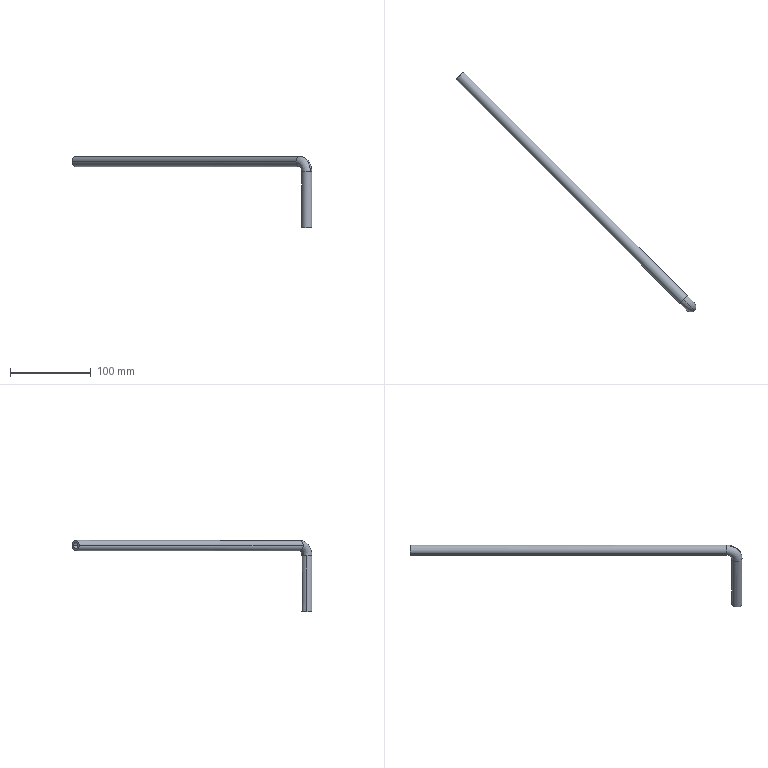Part | STEP file | Tube-500X095_3^Tube_6-P01_ASSEMBLY_KOMBAJN_OWOCOWY-003V11_Tube .500in OD X .095in Wall | 1 solid | 14 faces | box 297.218 x 297.218 x 88.076 mm | volume 37531 mm3 | cylinder 8 | torus 4 | plane 2 | commonest cylinder face diameters 7.874 x4 12.7 x4
STEP:
#1=CARTESIAN_POINT('',(0.,0.,0.));
#2=DIRECTION('',(0.,0.,1.));
#3=DIRECTION('',(1.,0.,0.));
#4=AXIS2_PLACEMENT_3D('',#1,#2,#3);
#5=CARTESIAN_POINT('',(3.937,0.,69.026));
#6=VERTEX_POINT('',#5);
#7=CARTESIAN_POINT('',(-2.784,2.784,69.026));
#8=VERTEX_POINT('',#7);
#9=CARTESIAN_POINT('',(0.,0.,69.026));
#10=DIRECTION('',(0.,0.,1.));
#11=DIRECTION('',(0.,1.,0.));
#12=AXIS2_PLACEMENT_3D('',#9,#10,#11);
#13=CIRCLE('',#12,3.937);
#14=CARTESIAN_POINT('',(-8.98,8.98,69.026));
#15=DIRECTION('',(-0.7071,-0.7071,0.));
#16=DIRECTION('',(0.7071,-0.7071,0.));
#17=AXIS2_PLACEMENT_3D('',#14,#15,#16);
#18=TOROIDAL_SURFACE('',#17,12.7,3.937);
#19=CARTESIAN_POINT('',(0.,10.21));
#20=DIRECTION('',(0.,-1.));
#21=VECTOR('',#20,1.);
#22=LINE('',#19,#21);
#23=(GEOMETRIC_REPRESENTATION_CONTEXT(2)PARAMETRIC_REPRESENTATION_CONTEXT()REPRESENTATION_CONTEXT('',''));
#24=DEFINITIONAL_REPRESENTATION('',(#22),#23);
#25=PCURVE('',#18,#24);
#26=CARTESIAN_POINT('',(0.,0.,69.026));
#27=DIRECTION('',(0.,0.,-1.));
#28=DIRECTION('',(-1.,0.,0.));
#29=AXIS2_PLACEMENT_3D('',#26,#27,#28);
#30=CYLINDRICAL_SURFACE('',#29,3.937);
#31=CARTESIAN_POINT('',(7.854,0.));
#32=DIRECTION('',(-1.,0.));
#33=VECTOR('',#32,1.);
#34=LINE('',#31,#33);
#35=(GEOMETRIC_REPRESENTATION_CONTEXT(2)PARAMETRIC_REPRESENTATION_CONTEXT()REPRESENTATION_CONTEXT('',''));
#36=DEFINITIONAL_REPRESENTATION('',(#34),#35);
#37=PCURVE('',#30,#36);
#38=SURFACE_CURVE('',#13,(#25,#37),.PCURVE_S1.);
#39=EDGE_CURVE('',#6,#8,#38,.T.);
#40=ORIENTED_EDGE('',*,*,#39,.T.);
#41=CARTESIAN_POINT('',(-8.98,8.98,77.789));
#42=VERTEX_POINT('',#41);
#43=CARTESIAN_POINT('',(-8.98,8.98,69.026));
#44=DIRECTION('',(-0.7071,-0.7071,0.));
#45=DIRECTION('',(0.7071,-0.7071,0.));
#46=AXIS2_PLACEMENT_3D('',#43,#44,#45);
#47=CIRCLE('',#46,8.763);
#48=CARTESIAN_POINT('',(0.,3.142));
#49=DIRECTION('',(1.,0.));
#50=VECTOR('',#49,1.);
#51=LINE('',#48,#50);
#52=(GEOMETRIC_REPRESENTATION_CONTEXT(2)PARAMETRIC_REPRESENTATION_CONTEXT()REPRESENTATION_CONTEXT('',''));
#53=DEFINITIONAL_REPRESENTATION('',(#51),#52);
#54=PCURVE('',#18,#53);
#55=CARTESIAN_POINT('',(-8.98,8.98,69.026));
#56=DIRECTION('',(-0.7071,-0.7071,0.));
#57=DIRECTION('',(0.7071,-0.7071,0.));
#58=AXIS2_PLACEMENT_3D('',#55,#56,#57);
#59=TOROIDAL_SURFACE('',#58,12.7,3.937);
#60=CARTESIAN_POINT('',(0.,3.142));
#61=DIRECTION('',(1.,0.));
#62=VECTOR('',#61,1.);
#63=LINE('',#60,#62);
#64=(GEOMETRIC_REPRESENTATION_CONTEXT(2)PARAMETRIC_REPRESENTATION_CONTEXT()REPRESENTATION_CONTEXT('',''));
#65=DEFINITIONAL_REPRESENTATION('',(#63),#64);
#66=PCURVE('',#59,#65);
#67=SURFACE_CURVE('',#47,(#54,#66),.PCURVE_S1.);
#68=EDGE_CURVE('',#8,#42,#67,.T.);
#69=ORIENTED_EDGE('',*,*,#68,.T.);
#70=CARTESIAN_POINT('',(-6.196,11.764,81.726));
#71=VERTEX_POINT('',#70);
#72=CARTESIAN_POINT('',(-8.98,8.98,81.726));
#73=DIRECTION('',(-0.7071,0.7071,0.));
#74=DIRECTION('',(-0.7071,-0.7071,0.));
#75=AXIS2_PLACEMENT_3D('',#72,#73,#74);
#76=CIRCLE('',#75,3.937);
#77=CARTESIAN_POINT('',(1.571,7.854));
#78=DIRECTION('',(0.,-1.));
#79=VECTOR('',#78,1.);
#80=LINE('',#77,#79);
#81=(GEOMETRIC_REPRESENTATION_CONTEXT(2)PARAMETRIC_REPRESENTATION_CONTEXT()REPRESENTATION_CONTEXT('',''));
#82=DEFINITIONAL_REPRESENTATION('',(#80),#81);
#83=PCURVE('',#18,#82);
#84=CARTESIAN_POINT('',(-8.98,8.98,81.726));
#85=DIRECTION('',(-0.7071,0.7071,0.));
#86=DIRECTION('',(-0.7071,-0.7071,0.));
#87=AXIS2_PLACEMENT_3D('',#84,#85,#86);
#88=CYLINDRICAL_SURFACE('',#87,3.937);
#89=CARTESIAN_POINT('',(0.,0.));
#90=DIRECTION('',(1.,0.));
#91=VECTOR('',#90,1.);
#92=LINE('',#89,#91);
#93=(GEOMETRIC_REPRESENTATION_CONTEXT(2)PARAMETRIC_REPRESENTATION_CONTEXT()REPRESENTATION_CONTEXT('',''));
#94=DEFINITIONAL_REPRESENTATION('',(#92),#93);
#95=PCURVE('',#88,#94);
#96=SURFACE_CURVE('',#76,(#83,#95),.PCURVE_S1.);
#97=EDGE_CURVE('',#71,#42,#96,.T.);
#98=ORIENTED_EDGE('',*,*,#97,.F.);
#99=CARTESIAN_POINT('',(-8.98,8.98,85.663));
#100=VERTEX_POINT('',#99);
#101=CARTESIAN_POINT('',(-8.98,8.98,81.726));
#102=DIRECTION('',(-0.7071,0.7071,0.));
#103=DIRECTION('',(-0.7071,-0.7071,0.));
#104=AXIS2_PLACEMENT_3D('',#101,#102,#103);
#105=CIRCLE('',#104,3.937);
#106=CARTESIAN_POINT('',(1.571,7.854));
#107=DIRECTION('',(0.,-1.));
#108=VECTOR('',#107,1.);
#109=LINE('',#106,#108);
#110=(GEOMETRIC_REPRESENTATION_CONTEXT(2)PARAMETRIC_REPRESENTATION_CONTEXT()REPRESENTATION_CONTEXT('',''));
#111=DEFINITIONAL_REPRESENTATION('',(#109),#110);
#112=PCURVE('',#18,#111);
#113=CARTESIAN_POINT('',(-8.98,8.98,81.726));
#114=DIRECTION('',(-0.7071,0.7071,0.));
#115=DIRECTION('',(-0.7071,-0.7071,0.));
#116=AXIS2_PLACEMENT_3D('',#113,#114,#115);
#117=CYLINDRICAL_SURFACE('',#116,3.937);
#118=CARTESIAN_POINT('',(0.,0.));
#119=DIRECTION('',(1.,0.));
#120=VECTOR('',#119,1.);
#121=LINE('',#118,#120);
#122=(GEOMETRIC_REPRESENTATION_CONTEXT(2)PARAMETRIC_REPRESENTATION_CONTEXT()REPRESENTATION_CONTEXT('',''));
#123=DEFINITIONAL_REPRESENTATION('',(#121),#122);
#124=PCURVE('',#117,#123);
#125=SURFACE_CURVE('',#105,(#112,#124),.PCURVE_S1.);
#126=EDGE_CURVE('',#100,#71,#125,.T.);
#127=ORIENTED_EDGE('',*,*,#126,.F.);
#128=CARTESIAN_POINT('',(2.784,-2.784,69.026));
#129=VERTEX_POINT('',#128);
#130=CARTESIAN_POINT('',(-8.98,8.98,69.026));
#131=DIRECTION('',(-0.7071,-0.7071,0.));
#132=DIRECTION('',(0.7071,-0.7071,0.));
#133=AXIS2_PLACEMENT_3D('',#130,#131,#132);
#134=CIRCLE('',#133,16.637);
#135=CARTESIAN_POINT('',(0.,6.283));
#136=DIRECTION('',(1.,0.));
#137=VECTOR('',#136,1.);
#138=LINE('',#135,#137);
#139=(GEOMETRIC_REPRESENTATION_CONTEXT(2)PARAMETRIC_REPRESENTATION_CONTEXT()REPRESENTATION_CONTEXT('',''));
#140=DEFINITIONAL_REPRESENTATION('',(#138),#139);
#141=PCURVE('',#18,#140);
#142=CARTESIAN_POINT('',(0.,0.));
#143=DIRECTION('',(1.,0.));
#144=VECTOR('',#143,1.);
#145=LINE('',#142,#144);
#146=(GEOMETRIC_REPRESENTATION_CONTEXT(2)PARAMETRIC_REPRESENTATION_CONTEXT()REPRESENTATION_CONTEXT('',''));
#147=DEFINITIONAL_REPRESENTATION('',(#145),#146);
#148=PCURVE('',#59,#147);
#149=SURFACE_CURVE('',#134,(#141,#148),.PCURVE_S1.);
#150=EDGE_CURVE('',#129,#100,#149,.T.);
#151=ORIENTED_EDGE('',*,*,#150,.F.);
#152=CARTESIAN_POINT('',(0.,0.,69.026));
#153=DIRECTION('',(0.,0.,1.));
#154=DIRECTION('',(0.,1.,0.));
#155=AXIS2_PLACEMENT_3D('',#152,#153,#154);
#156=CIRCLE('',#155,3.937);
#157=CARTESIAN_POINT('',(0.,10.21));
#158=DIRECTION('',(0.,-1.));
#159=VECTOR('',#158,1.);
#160=LINE('',#157,#159);
#161=(GEOMETRIC_REPRESENTATION_CONTEXT(2)PARAMETRIC_REPRESENTATION_CONTEXT()REPRESENTATION_CONTEXT('',''));
#162=DEFINITIONAL_REPRESENTATION('',(#160),#161);
#163=PCURVE('',#18,#162);
#164=CARTESIAN_POINT('',(0.,0.,69.026));
#165=DIRECTION('',(0.,0.,-1.));
#166=DIRECTION('',(-1.,0.,0.));
#167=AXIS2_PLACEMENT_3D('',#164,#165,#166);
#168=CYLINDRICAL_SURFACE('',#167,3.937);
#169=CARTESIAN_POINT('',(7.854,0.));
#170=DIRECTION('',(-1.,0.));
#171=VECTOR('',#170,1.);
#172=LINE('',#169,#171);
#173=(GEOMETRIC_REPRESENTATION_CONTEXT(2)PARAMETRIC_REPRESENTATION_CONTEXT()REPRESENTATION_CONTEXT('',''));
#174=DEFINITIONAL_REPRESENTATION('',(#172),#173);
#175=PCURVE('',#168,#174);
#176=SURFACE_CURVE('',#156,(#163,#175),.PCURVE_S1.);
#177=EDGE_CURVE('',#129,#6,#176,.T.);
#178=ORIENTED_EDGE('',*,*,#177,.T.);
#179=EDGE_LOOP('',(#40,#69,#98,#127,#151,#178));
#180=FACE_BOUND('',#179,.F.);
#181=ADVANCED_FACE('',(#180),#18,.F.);
#182=CARTESIAN_POINT('',(-6.35,0.,69.026));
#183=VERTEX_POINT('',#182);
#184=CARTESIAN_POINT('',(4.49,-4.49,69.026));
#185=VERTEX_POINT('',#184);
#186=CARTESIAN_POINT('',(0.,0.,69.026));
#187=DIRECTION('',(0.,0.,1.));
#188=DIRECTION('',(1.,0.,0.));
#189=AXIS2_PLACEMENT_3D('',#186,#187,#188);
#190=CIRCLE('',#189,6.35);
#191=CARTESIAN_POINT('',(-8.98,8.98,69.026));
#192=DIRECTION('',(-0.7071,-0.7071,0.));
#193=DIRECTION('',(0.7071,-0.7071,0.));
#194=AXIS2_PLACEMENT_3D('',#191,#192,#193);
#195=TOROIDAL_SURFACE('',#194,12.7,6.35);
#196=CARTESIAN_POINT('',(0.,5.498));
#197=DIRECTION('',(0.,-1.));
#198=VECTOR('',#197,1.);
#199=LINE('',#196,#198);
#200=(GEOMETRIC_REPRESENTATION_CONTEXT(2)PARAMETRIC_REPRESENTATION_CONTEXT()REPRESENTATION_CONTEXT('',''));
#201=DEFINITIONAL_REPRESENTATION('',(#199),#200);
#202=PCURVE('',#195,#201);
#203=CARTESIAN_POINT('',(0.,0.,69.026));
#204=DIRECTION('',(0.,0.,-1.));
#205=DIRECTION('',(-1.,0.,0.));
#206=AXIS2_PLACEMENT_3D('',#203,#204,#205);
#207=CYLINDRICAL_SURFACE('',#206,6.35);
#208=CARTESIAN_POINT('',(9.425,0.));
#209=DIRECTION('',(-1.,0.));
#210=VECTOR('',#209,1.);
#211=LINE('',#208,#210);
#212=(GEOMETRIC_REPRESENTATION_CONTEXT(2)PARAMETRIC_REPRESENTATION_CONTEXT()REPRESENTATION_CONTEXT('',''));
#213=DEFINITIONAL_REPRESENTATION('',(#211),#212);
#214=PCURVE('',#207,#213);
#215=SURFACE_CURVE('',#190,(#202,#214),.PCURVE_S1.);
#216=EDGE_CURVE('',#183,#185,#215,.T.);
#217=ORIENTED_EDGE('',*,*,#216,.T.);
#218=CARTESIAN_POINT('',(-8.98,8.98,88.076));
#219=VERTEX_POINT('',#218);
#220=CARTESIAN_POINT('',(-8.98,8.98,69.026));
#221=DIRECTION('',(-0.7071,-0.7071,0.));
#222=DIRECTION('',(0.7071,-0.7071,0.));
#223=AXIS2_PLACEMENT_3D('',#220,#221,#222);
#224=CIRCLE('',#223,19.05);
#225=CARTESIAN_POINT('',(0.,0.));
#226=DIRECTION('',(1.,0.));
#227=VECTOR('',#226,1.);
#228=LINE('',#225,#227);
#229=(GEOMETRIC_REPRESENTATION_CONTEXT(2)PARAMETRIC_REPRESENTATION_CONTEXT()REPRESENTATION_CONTEXT('',''));
#230=DEFINITIONAL_REPRESENTATION('',(#228),#229);
#231=PCURVE('',#195,#230);
#232=CARTESIAN_POINT('',(-8.98,8.98,69.026));
#233=DIRECTION('',(-0.7071,-0.7071,0.));
#234=DIRECTION('',(0.7071,-0.7071,0.));
#235=AXIS2_PLACEMENT_3D('',#232,#233,#234);
#236=TOROIDAL_SURFACE('',#235,12.7,6.35);
#237=CARTESIAN_POINT('',(0.,6.283));
#238=DIRECTION('',(1.,0.));
#239=VECTOR('',#238,1.);
#240=LINE('',#237,#239);
#241=(GEOMETRIC_REPRESENTATION_CONTEXT(2)PARAMETRIC_REPRESENTATION_CONTEXT()REPRESENTATION_CONTEXT('',''));
#242=DEFINITIONAL_REPRESENTATION('',(#240),#241);
#243=PCURVE('',#236,#242);
#244=SURFACE_CURVE('',#224,(#231,#243),.PCURVE_S1.);
#245=EDGE_CURVE('',#185,#219,#244,.T.);
#246=ORIENTED_EDGE('',*,*,#245,.T.);
#247=CARTESIAN_POINT('',(-13.47,4.49,81.726));
#248=VERTEX_POINT('',#247);
#249=CARTESIAN_POINT('',(-8.98,8.98,81.726));
#250=DIRECTION('',(-0.7071,0.7071,0.));
#251=DIRECTION('',(0.5,0.5,0.7071));
#252=AXIS2_PLACEMENT_3D('',#249,#250,#251);
#253=CIRCLE('',#252,6.35);
#254=CARTESIAN_POINT('',(1.571,5.498));
#255=DIRECTION('',(0.,-1.));
#256=VECTOR('',#255,1.);
#257=LINE('',#254,#256);
#258=(GEOMETRIC_REPRESENTATION_CONTEXT(2)PARAMETRIC_REPRESENTATION_CONTEXT()REPRESENTATION_CONTEXT('',''));
#259=DEFINITIONAL_REPRESENTATION('',(#257),#258);
#260=PCURVE('',#195,#259);
#261=CARTESIAN_POINT('',(-8.98,8.98,81.726));
#262=DIRECTION('',(-0.7071,0.7071,0.));
#263=DIRECTION('',(-0.7071,-0.7071,0.));
#264=AXIS2_PLACEMENT_3D('',#261,#262,#263);
#265=CYLINDRICAL_SURFACE('',#264,6.35);
#266=CARTESIAN_POINT('',(-3.927,0.));
#267=DIRECTION('',(1.,0.));
#268=VECTOR('',#267,1.);
#269=LINE('',#266,#268);
#270=(GEOMETRIC_REPRESENTATION_CONTEXT(2)PARAMETRIC_REPRESENTATION_CONTEXT()REPRESENTATION_CONTEXT('',''));
#271=DEFINITIONAL_REPRESENTATION('',(#269),#270);
#272=PCURVE('',#265,#271);
#273=SURFACE_CURVE('',#253,(#260,#272),.PCURVE_S1.);
#274=EDGE_CURVE('',#248,#219,#273,.T.);
#275=ORIENTED_EDGE('',*,*,#274,.F.);
#276=CARTESIAN_POINT('',(-8.98,8.98,75.376));
#277=VERTEX_POINT('',#276);
#278=CARTESIAN_POINT('',(-8.98,8.98,81.726));
#279=DIRECTION('',(-0.7071,0.7071,0.));
#280=DIRECTION('',(0.5,0.5,0.7071));
#281=AXIS2_PLACEMENT_3D('',#278,#279,#280);
#282=CIRCLE('',#281,6.35);
#283=CARTESIAN_POINT('',(1.571,5.498));
#284=DIRECTION('',(0.,-1.));
#285=VECTOR('',#284,1.);
#286=LINE('',#283,#285);
#287=(GEOMETRIC_REPRESENTATION_CONTEXT(2)PARAMETRIC_REPRESENTATION_CONTEXT()REPRESENTATION_CONTEXT('',''));
#288=DEFINITIONAL_REPRESENTATION('',(#286),#287);
#289=PCURVE('',#195,#288);
#290=CARTESIAN_POINT('',(-8.98,8.98,81.726));
#291=DIRECTION('',(-0.7071,0.7071,0.));
#292=DIRECTION('',(-0.7071,-0.7071,0.));
#293=AXIS2_PLACEMENT_3D('',#290,#291,#292);
#294=CYLINDRICAL_SURFACE('',#293,6.35);
#295=CARTESIAN_POINT('',(2.356,0.));
#296=DIRECTION('',(1.,0.));
#297=VECTOR('',#296,1.);
#298=LINE('',#295,#297);
#299=(GEOMETRIC_REPRESENTATION_CONTEXT(2)PARAMETRIC_REPRESENTATION_CONTEXT()REPRESENTATION_CONTEXT('',''));
#300=DEFINITIONAL_REPRESENTATION('',(#298),#299);
#301=PCURVE('',#294,#300);
#302=SURFACE_CURVE('',#282,(#289,#301),.PCURVE_S1.);
#303=EDGE_CURVE('',#277,#248,#302,.T.);
#304=ORIENTED_EDGE('',*,*,#303,.F.);
#305=CARTESIAN_POINT('',(-4.49,4.49,69.026));
#306=VERTEX_POINT('',#305);
#307=CARTESIAN_POINT('',(-8.98,8.98,69.026));
#308=DIRECTION('',(-0.7071,-0.7071,0.));
#309=DIRECTION('',(0.7071,-0.7071,0.));
#310=AXIS2_PLACEMENT_3D('',#307,#308,#309);
#311=CIRCLE('',#310,6.35);
#312=CARTESIAN_POINT('',(0.,3.142));
#313=DIRECTION('',(1.,0.));
#314=VECTOR('',#313,1.);
#315=LINE('',#312,#314);
#316=(GEOMETRIC_REPRESENTATION_CONTEXT(2)PARAMETRIC_REPRESENTATION_CONTEXT()REPRESENTATION_CONTEXT('',''));
#317=DEFINITIONAL_REPRESENTATION('',(#315),#316);
#318=PCURVE('',#195,#317);
#319=CARTESIAN_POINT('',(0.,3.142));
#320=DIRECTION('',(1.,0.));
#321=VECTOR('',#320,1.);
#322=LINE('',#319,#321);
#323=(GEOMETRIC_REPRESENTATION_CONTEXT(2)PARAMETRIC_REPRESENTATION_CONTEXT()REPRESENTATION_CONTEXT('',''));
#324=DEFINITIONAL_REPRESENTATION('',(#322),#323);
#325=PCURVE('',#236,#324);
#326=SURFACE_CURVE('',#311,(#318,#325),.PCURVE_S1.);
#327=EDGE_CURVE('',#306,#277,#326,.T.);
#328=ORIENTED_EDGE('',*,*,#327,.F.);
#329=CARTESIAN_POINT('',(0.,0.,69.026));
#330=DIRECTION('',(0.,0.,1.));
#331=DIRECTION('',(1.,0.,0.));
#332=AXIS2_PLACEMENT_3D('',#329,#330,#331);
#333=CIRCLE('',#332,6.35);
#334=CARTESIAN_POINT('',(0.,5.498));
#335=DIRECTION('',(0.,-1.));
#336=VECTOR('',#335,1.);
#337=LINE('',#334,#336);
#338=(GEOMETRIC_REPRESENTATION_CONTEXT(2)PARAMETRIC_REPRESENTATION_CONTEXT()REPRESENTATION_CONTEXT('',''));
#339=DEFINITIONAL_REPRESENTATION('',(#337),#338);
#340=PCURVE('',#195,#339);
#341=CARTESIAN_POINT('',(0.,0.,69.026));
#342=DIRECTION('',(0.,0.,-1.));
#343=DIRECTION('',(-1.,0.,0.));
#344=AXIS2_PLACEMENT_3D('',#341,#342,#343);
#345=CYLINDRICAL_SURFACE('',#344,6.35);
#346=CARTESIAN_POINT('',(3.142,0.));
#347=DIRECTION('',(-1.,0.));
#348=VECTOR('',#347,1.);
#349=LINE('',#346,#348);
#350=(GEOMETRIC_REPRESENTATION_CONTEXT(2)PARAMETRIC_REPRESENTATION_CONTEXT()REPRESENTATION_CONTEXT('',''));
#351=DEFINITIONAL_REPRESENTATION('',(#349),#350);
#352=PCURVE('',#345,#351);
#353=SURFACE_CURVE('',#333,(#340,#352),.PCURVE_S1.);
#354=EDGE_CURVE('',#306,#183,#353,.T.);
#355=ORIENTED_EDGE('',*,*,#354,.T.);
#356=EDGE_LOOP('',(#217,#246,#275,#304,#328,#355));
#357=FACE_BOUND('',#356,.T.);
#358=ADVANCED_FACE('',(#357),#195,.T.);
#359=CARTESIAN_POINT('',(-3.937,0.,69.026));
#360=VERTEX_POINT('',#359);
#361=CARTESIAN_POINT('',(-3.937,0.,0.));
#362=VERTEX_POINT('',#361);
#363=CARTESIAN_POINT('',(-3.937,0.,69.026));
#364=DIRECTION('',(0.,0.,-1.));
#365=VECTOR('',#364,1.);
#366=LINE('',#363,#365);
#367=CARTESIAN_POINT('',(6.283,0.));
#368=DIRECTION('',(0.,1.));
#369=VECTOR('',#368,1.);
#370=LINE('',#367,#369);
#371=(GEOMETRIC_REPRESENTATION_CONTEXT(2)PARAMETRIC_REPRESENTATION_CONTEXT()REPRESENTATION_CONTEXT('',''));
#372=DEFINITIONAL_REPRESENTATION('',(#370),#371);
#373=PCURVE('',#168,#372);
#374=CARTESIAN_POINT('',(0.,0.));
#375=DIRECTION('',(0.,1.));
#376=VECTOR('',#375,1.);
#377=LINE('',#374,#376);
#378=(GEOMETRIC_REPRESENTATION_CONTEXT(2)PARAMETRIC_REPRESENTATION_CONTEXT()REPRESENTATION_CONTEXT('',''));
#379=DEFINITIONAL_REPRESENTATION('',(#377),#378);
#380=PCURVE('',#30,#379);
#381=SURFACE_CURVE('',#366,(#373,#380),.PCURVE_S1.);
#382=EDGE_CURVE('',#360,#362,#381,.T.);
#383=ORIENTED_EDGE('',*,*,#382,.T.);
#384=CARTESIAN_POINT('',(3.937,0.,0.));
#385=VERTEX_POINT('',#384);
#386=CARTESIAN_POINT('',(0.,0.,0.));
#387=DIRECTION('',(0.,0.,1.));
#388=DIRECTION('',(1.,0.,0.));
#389=AXIS2_PLACEMENT_3D('',#386,#387,#388);
#390=CIRCLE('',#389,3.937);
#391=CARTESIAN_POINT('',(9.425,69.026));
#392=DIRECTION('',(-1.,0.));
#393=VECTOR('',#392,1.);
#394=LINE('',#391,#393);
#395=(GEOMETRIC_REPRESENTATION_CONTEXT(2)PARAMETRIC_REPRESENTATION_CONTEXT()REPRESENTATION_CONTEXT('',''));
#396=DEFINITIONAL_REPRESENTATION('',(#394),#395);
#397=PCURVE('',#168,#396);
#398=CARTESIAN_POINT('',(0.,0.,0.));
#399=DIRECTION('',(0.,0.,1.));
#400=DIRECTION('',(1.,0.,0.));
#401=AXIS2_PLACEMENT_3D('',#398,#399,#400);
#402=PLANE('',#401);
#403=CARTESIAN_POINT('',(0.,0.));
#404=DIRECTION('',(1.,0.));
#405=AXIS2_PLACEMENT_2D('',#403,#404);
#406=CIRCLE('',#405,3.937);
#407=(GEOMETRIC_REPRESENTATION_CONTEXT(2)PARAMETRIC_REPRESENTATION_CONTEXT()REPRESENTATION_CONTEXT('',''));
#408=DEFINITIONAL_REPRESENTATION('',(#406),#407);
#409=PCURVE('',#402,#408);
#410=SURFACE_CURVE('',#390,(#397,#409),.PCURVE_S1.);
#411=EDGE_CURVE('',#362,#385,#410,.T.);
#412=ORIENTED_EDGE('',*,*,#411,.T.);
#413=CARTESIAN_POINT('',(3.937,0.,69.026));
#414=DIRECTION('',(0.,0.,-1.));
#415=VECTOR('',#414,1.);
#416=LINE('',#413,#415);
#417=CARTESIAN_POINT('',(3.142,0.));
#418=DIRECTION('',(0.,1.));
#419=VECTOR('',#418,1.);
#420=LINE('',#417,#419);
#421=(GEOMETRIC_REPRESENTATION_CONTEXT(2)PARAMETRIC_REPRESENTATION_CONTEXT()REPRESENTATION_CONTEXT('',''));
#422=DEFINITIONAL_REPRESENTATION('',(#420),#421);
#423=PCURVE('',#168,#422);
#424=CARTESIAN_POINT('',(3.142,0.));
#425=DIRECTION('',(0.,1.));
#426=VECTOR('',#425,1.);
#427=LINE('',#424,#426);
#428=(GEOMETRIC_REPRESENTATION_CONTEXT(2)PARAMETRIC_REPRESENTATION_CONTEXT()REPRESENTATION_CONTEXT('',''));
#429=DEFINITIONAL_REPRESENTATION('',(#427),#428);
#430=PCURVE('',#30,#429);
#431=SURFACE_CURVE('',#416,(#423,#430),.PCURVE_S1.);
#432=EDGE_CURVE('',#6,#385,#431,.T.);
#433=ORIENTED_EDGE('',*,*,#432,.F.);
#434=ORIENTED_EDGE('',*,*,#177,.F.);
#435=CARTESIAN_POINT('',(0.,0.,69.026));
#436=DIRECTION('',(0.,0.,1.));
#437=DIRECTION('',(0.,1.,0.));
#438=AXIS2_PLACEMENT_3D('',#435,#436,#437);
#439=CIRCLE('',#438,3.937);
#440=CARTESIAN_POINT('',(7.854,0.));
#441=DIRECTION('',(-1.,0.));
#442=VECTOR('',#441,1.);
#443=LINE('',#440,#442);
#444=(GEOMETRIC_REPRESENTATION_CONTEXT(2)PARAMETRIC_REPRESENTATION_CONTEXT()REPRESENTATION_CONTEXT('',''));
#445=DEFINITIONAL_REPRESENTATION('',(#443),#444);
#446=PCURVE('',#168,#445);
#447=CARTESIAN_POINT('',(0.,3.927));
#448=DIRECTION('',(0.,-1.));
#449=VECTOR('',#448,1.);
#450=LINE('',#447,#449);
#451=(GEOMETRIC_REPRESENTATION_CONTEXT(2)PARAMETRIC_REPRESENTATION_CONTEXT()REPRESENTATION_CONTEXT('',''));
#452=DEFINITIONAL_REPRESENTATION('',(#450),#451);
#453=PCURVE('',#59,#452);
#454=SURFACE_CURVE('',#439,(#446,#453),.PCURVE_S1.);
#455=EDGE_CURVE('',#360,#129,#454,.T.);
#456=ORIENTED_EDGE('',*,*,#455,.F.);
#457=EDGE_LOOP('',(#383,#412,#433,#434,#456));
#458=FACE_BOUND('',#457,.F.);
#459=ADVANCED_FACE('',(#458),#168,.F.);
#460=CARTESIAN_POINT('',(-11.764,6.196,81.726));
#461=VERTEX_POINT('',#460);
#462=CARTESIAN_POINT('',(-8.98,8.98,81.726));
#463=DIRECTION('',(-0.7071,0.7071,0.));
#464=DIRECTION('',(-0.7071,-0.7071,0.));
#465=AXIS2_PLACEMENT_3D('',#462,#463,#464);
#466=CIRCLE('',#465,3.937);
#467=CARTESIAN_POINT('',(0.,0.));
#468=DIRECTION('',(1.,0.));
#469=VECTOR('',#468,1.);
#470=LINE('',#467,#469);
#471=(GEOMETRIC_REPRESENTATION_CONTEXT(2)PARAMETRIC_REPRESENTATION_CONTEXT()REPRESENTATION_CONTEXT('',''));
#472=DEFINITIONAL_REPRESENTATION('',(#470),#471);
#473=PCURVE('',#88,#472);
#474=CARTESIAN_POINT('',(1.571,7.854));
#475=DIRECTION('',(0.,-1.));
#476=VECTOR('',#475,1.);
#477=LINE('',#474,#476);
#478=(GEOMETRIC_REPRESENTATION_CONTEXT(2)PARAMETRIC_REPRESENTATION_CONTEXT()REPRESENTATION_CONTEXT('',''));
#479=DEFINITIONAL_REPRESENTATION('',(#477),#478);
#480=PCURVE('',#59,#479);
#481=SURFACE_CURVE('',#466,(#473,#480),.PCURVE_S1.);
#482=EDGE_CURVE('',#42,#461,#481,.T.);
#483=ORIENTED_EDGE('',*,*,#482,.T.);
#484=CARTESIAN_POINT('',(-289.161,283.594,81.726));
#485=VERTEX_POINT('',#484);
#486=CARTESIAN_POINT('',(-11.764,6.196,81.726));
#487=DIRECTION('',(-0.7071,0.7071,0.));
#488=VECTOR('',#487,1.);
#489=LINE('',#486,#488);
#490=CARTESIAN_POINT('',(6.283,0.));
#491=DIRECTION('',(0.,1.));
#492=VECTOR('',#491,1.);
#493=LINE('',#490,#492);
#494=(GEOMETRIC_REPRESENTATION_CONTEXT(2)PARAMETRIC_REPRESENTATION_CONTEXT()REPRESENTATION_CONTEXT('',''));
#495=DEFINITIONAL_REPRESENTATION('',(#493),#494);
#496=PCURVE('',#88,#495);
#497=CARTESIAN_POINT('',(0.,0.));
#498=DIRECTION('',(0.,1.));
#499=VECTOR('',#498,1.);
#500=LINE('',#497,#499);
#501=(GEOMETRIC_REPRESENTATION_CONTEXT(2)PARAMETRIC_REPRESENTATION_CONTEXT()REPRESENTATION_CONTEXT('',''));
#502=DEFINITIONAL_REPRESENTATION('',(#500),#501);
#503=PCURVE('',#117,#502);
#504=SURFACE_CURVE('',#489,(#496,#503),.PCURVE_S1.);
#505=EDGE_CURVE('',#461,#485,#504,.T.);
#506=ORIENTED_EDGE('',*,*,#505,.T.);
#507=CARTESIAN_POINT('',(-283.594,289.161,81.726));
#508=VERTEX_POINT('',#507);
#509=CARTESIAN_POINT('',(-286.377,286.377,81.726));
#510=DIRECTION('',(-0.7071,0.7071,0.));
#511=DIRECTION('',(-0.7071,-0.7071,0.));
#512=AXIS2_PLACEMENT_3D('',#509,#510,#511);
#513=CIRCLE('',#512,3.937);
#514=CARTESIAN_POINT('',(0.,392.299));
#515=DIRECTION('',(1.,0.));
#516=VECTOR('',#515,1.);
#517=LINE('',#514,#516);
#518=(GEOMETRIC_REPRESENTATION_CONTEXT(2)PARAMETRIC_REPRESENTATION_CONTEXT()REPRESENTATION_CONTEXT('',''));
#519=DEFINITIONAL_REPRESENTATION('',(#517),#518);
#520=PCURVE('',#88,#519);
#521=CARTESIAN_POINT('',(-286.377,286.377,81.726));
#522=DIRECTION('',(-0.7071,0.7071,0.));
#523=DIRECTION('',(0.5,0.5,0.7071));
#524=AXIS2_PLACEMENT_3D('',#521,#522,#523);
#525=PLANE('',#524);
#526=CARTESIAN_POINT('',(0.,0.));
#527=DIRECTION('',(-0.7071,-0.7071));
#528=AXIS2_PLACEMENT_2D('',#526,#527);
#529=CIRCLE('',#528,3.937);
#530=(GEOMETRIC_REPRESENTATION_CONTEXT(2)PARAMETRIC_REPRESENTATION_CONTEXT()REPRESENTATION_CONTEXT('',''));
#531=DEFINITIONAL_REPRESENTATION('',(#529),#530);
#532=PCURVE('',#525,#531);
#533=SURFACE_CURVE('',#513,(#520,#532),.PCURVE_S1.);
#534=EDGE_CURVE('',#508,#485,#533,.T.);
#535=ORIENTED_EDGE('',*,*,#534,.F.);
#536=CARTESIAN_POINT('',(-6.196,11.764,81.726));
#537=DIRECTION('',(-0.7071,0.7071,0.));
#538=VECTOR('',#537,1.);
#539=LINE('',#536,#538);
#540=CARTESIAN_POINT('',(3.142,0.));
#541=DIRECTION('',(0.,1.));
#542=VECTOR('',#541,1.);
#543=LINE('',#540,#542);
#544=(GEOMETRIC_REPRESENTATION_CONTEXT(2)PARAMETRIC_REPRESENTATION_CONTEXT()REPRESENTATION_CONTEXT('',''));
#545=DEFINITIONAL_REPRESENTATION('',(#543),#544);
#546=PCURVE('',#88,#545);
#547=CARTESIAN_POINT('',(3.142,0.));
#548=DIRECTION('',(0.,1.));
#549=VECTOR('',#548,1.);
#550=LINE('',#547,#549);
#551=(GEOMETRIC_REPRESENTATION_CONTEXT(2)PARAMETRIC_REPRESENTATION_CONTEXT()REPRESENTATION_CONTEXT('',''));
#552=DEFINITIONAL_REPRESENTATION('',(#550),#551);
#553=PCURVE('',#117,#552);
#554=SURFACE_CURVE('',#539,(#546,#553),.PCURVE_S1.);
#555=EDGE_CURVE('',#71,#508,#554,.T.);
#556=ORIENTED_EDGE('',*,*,#555,.F.);
#557=ORIENTED_EDGE('',*,*,#97,.T.);
#558=EDGE_LOOP('',(#483,#506,#535,#556,#557));
#559=FACE_BOUND('',#558,.F.);
#560=ADVANCED_FACE('',(#559),#88,.F.);
#561=CARTESIAN_POINT('',(6.35,0.,69.026));
#562=VERTEX_POINT('',#561);
#563=CARTESIAN_POINT('',(0.,0.,69.026));
#564=DIRECTION('',(0.,0.,1.));
#565=DIRECTION('',(1.,0.,0.));
#566=AXIS2_PLACEMENT_3D('',#563,#564,#565);
#567=CIRCLE('',#566,6.35);
#568=CARTESIAN_POINT('',(3.142,0.));
#569=DIRECTION('',(-1.,0.));
#570=VECTOR('',#569,1.);
#571=LINE('',#568,#570);
#572=(GEOMETRIC_REPRESENTATION_CONTEXT(2)PARAMETRIC_REPRESENTATION_CONTEXT()REPRESENTATION_CONTEXT('',''));
#573=DEFINITIONAL_REPRESENTATION('',(#571),#572);
#574=PCURVE('',#345,#573);
#575=CARTESIAN_POINT('',(0.,5.498));
#576=DIRECTION('',(0.,-1.));
#577=VECTOR('',#576,1.);
#578=LINE('',#575,#577);
#579=(GEOMETRIC_REPRESENTATION_CONTEXT(2)PARAMETRIC_REPRESENTATION_CONTEXT()REPRESENTATION_CONTEXT('',''));
#580=DEFINITIONAL_REPRESENTATION('',(#578),#579);
#581=PCURVE('',#236,#580);
#582=SURFACE_CURVE('',#567,(#574,#581),.PCURVE_S1.);
#583=EDGE_CURVE('',#562,#306,#582,.T.);
#584=ORIENTED_EDGE('',*,*,#583,.F.);
#585=CARTESIAN_POINT('',(6.35,0.,0.));
#586=VERTEX_POINT('',#585);
#587=CARTESIAN_POINT('',(6.35,0.,69.026));
#588=DIRECTION('',(0.,0.,-1.));
#589=VECTOR('',#588,1.);
#590=LINE('',#587,#589);
#591=CARTESIAN_POINT('',(3.142,0.));
#592=DIRECTION('',(0.,1.));
#593=VECTOR('',#592,1.);
#594=LINE('',#591,#593);
#595=(GEOMETRIC_REPRESENTATION_CONTEXT(2)PARAMETRIC_REPRESENTATION_CONTEXT()REPRESENTATION_CONTEXT('',''));
#596=DEFINITIONAL_REPRESENTATION('',(#594),#595);
#597=PCURVE('',#345,#596);
#598=CARTESIAN_POINT('',(3.142,0.));
#599=DIRECTION('',(0.,1.));
#600=VECTOR('',#599,1.);
#601=LINE('',#598,#600);
#602=(GEOMETRIC_REPRESENTATION_CONTEXT(2)PARAMETRIC_REPRESENTATION_CONTEXT()REPRESENTATION_CONTEXT('',''));
#603=DEFINITIONAL_REPRESENTATION('',(#601),#602);
#604=PCURVE('',#207,#603);
#605=SURFACE_CURVE('',#590,(#597,#604),.PCURVE_S1.);
#606=EDGE_CURVE('',#562,#586,#605,.T.);
#607=ORIENTED_EDGE('',*,*,#606,.T.);
#608=CARTESIAN_POINT('',(-6.35,0.,0.));
#609=VERTEX_POINT('',#608);
#610=CARTESIAN_POINT('',(0.,0.,0.));
#611=DIRECTION('',(0.,0.,1.));
#612=DIRECTION('',(1.,0.,0.));
#613=AXIS2_PLACEMENT_3D('',#610,#611,#612);
#614=CIRCLE('',#613,6.35);
#615=CARTESIAN_POINT('',(3.142,69.026));
#616=DIRECTION('',(-1.,0.));
#617=VECTOR('',#616,1.);
#618=LINE('',#615,#617);
#619=(GEOMETRIC_REPRESENTATION_CONTEXT(2)PARAMETRIC_REPRESENTATION_CONTEXT()REPRESENTATION_CONTEXT('',''));
#620=DEFINITIONAL_REPRESENTATION('',(#618),#619);
#621=PCURVE('',#345,#620);
#622=CARTESIAN_POINT('',(0.,0.));
#623=DIRECTION('',(1.,0.));
#624=AXIS2_PLACEMENT_2D('',#622,#623);
#625=CIRCLE('',#624,6.35);
#626=(GEOMETRIC_REPRESENTATION_CONTEXT(2)PARAMETRIC_REPRESENTATION_CONTEXT()REPRESENTATION_CONTEXT('',''));
#627=DEFINITIONAL_REPRESENTATION('',(#625),#626);
#628=PCURVE('',#402,#627);
#629=SURFACE_CURVE('',#614,(#621,#628),.PCURVE_S1.);
#630=EDGE_CURVE('',#586,#609,#629,.T.);
#631=ORIENTED_EDGE('',*,*,#630,.T.);
#632=CARTESIAN_POINT('',(-6.35,0.,69.026));
#633=DIRECTION('',(0.,0.,-1.));
#634=VECTOR('',#633,1.);
#635=LINE('',#632,#634);
#636=CARTESIAN_POINT('',(0.,0.));
#637=DIRECTION('',(0.,1.));
#638=VECTOR('',#637,1.);
#639=LINE('',#636,#638);
#640=(GEOMETRIC_REPRESENTATION_CONTEXT(2)PARAMETRIC_REPRESENTATION_CONTEXT()REPRESENTATION_CONTEXT('',''));
#641=DEFINITIONAL_REPRESENTATION('',(#639),#640);
#642=PCURVE('',#345,#641);
#643=CARTESIAN_POINT('',(6.283,0.));
#644=DIRECTION('',(0.,1.));
#645=VECTOR('',#644,1.);
#646=LINE('',#643,#645);
#647=(GEOMETRIC_REPRESENTATION_CONTEXT(2)PARAMETRIC_REPRESENTATION_CONTEXT()REPRESENTATION_CONTEXT('',''));
#648=DEFINITIONAL_REPRESENTATION('',(#646),#647);
#649=PCURVE('',#207,#648);
#650=SURFACE_CURVE('',#635,(#642,#649),.PCURVE_S1.);
#651=EDGE_CURVE('',#183,#609,#650,.T.);
#652=ORIENTED_EDGE('',*,*,#651,.F.);
#653=ORIENTED_EDGE('',*,*,#354,.F.);
#654=EDGE_LOOP('',(#584,#607,#631,#652,#653));
#655=FACE_BOUND('',#654,.T.);
#656=ADVANCED_FACE('',(#655),#345,.T.);
#657=ORIENTED_EDGE('',*,*,#274,.T.);
#658=CARTESIAN_POINT('',(-4.49,13.47,81.726));
#659=VERTEX_POINT('',#658);
#660=CARTESIAN_POINT('',(-8.98,8.98,81.726));
#661=DIRECTION('',(-0.7071,0.7071,0.));
#662=DIRECTION('',(0.5,0.5,0.7071));
#663=AXIS2_PLACEMENT_3D('',#660,#661,#662);
#664=CIRCLE('',#663,6.35);
#665=CARTESIAN_POINT('',(-3.927,0.));
#666=DIRECTION('',(1.,0.));
#667=VECTOR('',#666,1.);
#668=LINE('',#665,#667);
#669=(GEOMETRIC_REPRESENTATION_CONTEXT(2)PARAMETRIC_REPRESENTATION_CONTEXT()REPRESENTATION_CONTEXT('',''));
#670=DEFINITIONAL_REPRESENTATION('',(#668),#669);
#671=PCURVE('',#265,#670);
#672=CARTESIAN_POINT('',(1.571,11.781));
#673=DIRECTION('',(0.,-1.));
#674=VECTOR('',#673,1.);
#675=LINE('',#672,#674);
#676=(GEOMETRIC_REPRESENTATION_CONTEXT(2)PARAMETRIC_REPRESENTATION_CONTEXT()REPRESENTATION_CONTEXT('',''));
#677=DEFINITIONAL_REPRESENTATION('',(#675),#676);
#678=PCURVE('',#236,#677);
#679=SURFACE_CURVE('',#664,(#671,#678),.PCURVE_S1.);
#680=EDGE_CURVE('',#219,#659,#679,.T.);
#681=ORIENTED_EDGE('',*,*,#680,.T.);
#682=CARTESIAN_POINT('',(-281.887,290.868,81.726));
#683=VERTEX_POINT('',#682);
#684=CARTESIAN_POINT('',(-4.49,13.47,81.726));
#685=DIRECTION('',(-0.7071,0.7071,0.));
#686=VECTOR('',#685,1.);
#687=LINE('',#684,#686);
#688=CARTESIAN_POINT('',(3.142,0.));
#689=DIRECTION('',(0.,1.));
#690=VECTOR('',#689,1.);
#691=LINE('',#688,#690);
#692=(GEOMETRIC_REPRESENTATION_CONTEXT(2)PARAMETRIC_REPRESENTATION_CONTEXT()REPRESENTATION_CONTEXT('',''));
#693=DEFINITIONAL_REPRESENTATION('',(#691),#692);
#694=PCURVE('',#265,#693);
#695=CARTESIAN_POINT('',(3.142,0.));
#696=DIRECTION('',(0.,1.));
#697=VECTOR('',#696,1.);
#698=LINE('',#695,#697);
#699=(GEOMETRIC_REPRESENTATION_CONTEXT(2)PARAMETRIC_REPRESENTATION_CONTEXT()REPRESENTATION_CONTEXT('',''));
#700=DEFINITIONAL_REPRESENTATION('',(#698),#699);
#701=PCURVE('',#294,#700);
#702=SURFACE_CURVE('',#687,(#694,#701),.PCURVE_S1.);
#703=EDGE_CURVE('',#659,#683,#702,.T.);
#704=ORIENTED_EDGE('',*,*,#703,.T.);
#705=CARTESIAN_POINT('',(-290.868,281.887,81.726));
#706=VERTEX_POINT('',#705);
#707=CARTESIAN_POINT('',(-286.377,286.377,81.726));
#708=DIRECTION('',(-0.7071,0.7071,0.));
#709=DIRECTION('',(0.5,0.5,0.7071));
#710=AXIS2_PLACEMENT_3D('',#707,#708,#709);
#711=CIRCLE('',#710,6.35);
#712=CARTESIAN_POINT('',(-3.927,392.299));
#713=DIRECTION('',(1.,0.));
#714=VECTOR('',#713,1.);
#715=LINE('',#712,#714);
#716=(GEOMETRIC_REPRESENTATION_CONTEXT(2)PARAMETRIC_REPRESENTATION_CONTEXT()REPRESENTATION_CONTEXT('',''));
#717=DEFINITIONAL_REPRESENTATION('',(#715),#716);
#718=PCURVE('',#265,#717);
#719=CARTESIAN_POINT('',(0.,0.));
#720=DIRECTION('',(1.,0.));
#721=AXIS2_PLACEMENT_2D('',#719,#720);
#722=CIRCLE('',#721,6.35);
#723=(GEOMETRIC_REPRESENTATION_CONTEXT(2)PARAMETRIC_REPRESENTATION_CONTEXT()REPRESENTATION_CONTEXT('',''));
#724=DEFINITIONAL_REPRESENTATION('',(#722),#723);
#725=PCURVE('',#525,#724);
#726=SURFACE_CURVE('',#711,(#718,#725),.PCURVE_S1.);
#727=EDGE_CURVE('',#706,#683,#726,.T.);
#728=ORIENTED_EDGE('',*,*,#727,.F.);
#729=CARTESIAN_POINT('',(-13.47,4.49,81.726));
#730=DIRECTION('',(-0.7071,0.7071,0.));
#731=VECTOR('',#730,1.);
#732=LINE('',#729,#731);
#733=CARTESIAN_POINT('',(0.,0.));
#734=DIRECTION('',(0.,1.));
#735=VECTOR('',#734,1.);
#736=LINE('',#733,#735);
#737=(GEOMETRIC_REPRESENTATION_CONTEXT(2)PARAMETRIC_REPRESENTATION_CONTEXT()REPRESENTATION_CONTEXT('',''));
#738=DEFINITIONAL_REPRESENTATION('',(#736),#737);
#739=PCURVE('',#265,#738);
#740=CARTESIAN_POINT('',(6.283,0.));
#741=DIRECTION('',(0.,1.));
#742=VECTOR('',#741,1.);
#743=LINE('',#740,#742);
#744=(GEOMETRIC_REPRESENTATION_CONTEXT(2)PARAMETRIC_REPRESENTATION_CONTEXT()REPRESENTATION_CONTEXT('',''));
#745=DEFINITIONAL_REPRESENTATION('',(#743),#744);
#746=PCURVE('',#294,#745);
#747=SURFACE_CURVE('',#732,(#739,#746),.PCURVE_S1.);
#748=EDGE_CURVE('',#248,#706,#747,.T.);
#749=ORIENTED_EDGE('',*,*,#748,.F.);
#750=EDGE_LOOP('',(#657,#681,#704,#728,#749));
#751=FACE_BOUND('',#750,.T.);
#752=ADVANCED_FACE('',(#751),#265,.T.);
#753=ORIENTED_EDGE('',*,*,#703,.F.);
#754=CARTESIAN_POINT('',(-8.98,8.98,81.726));
#755=DIRECTION('',(-0.7071,0.7071,0.));
#756=DIRECTION('',(0.5,0.5,0.7071));
#757=AXIS2_PLACEMENT_3D('',#754,#755,#756);
#758=CIRCLE('',#757,6.35);
#759=CARTESIAN_POINT('',(2.356,0.));
#760=DIRECTION('',(1.,0.));
#761=VECTOR('',#760,1.);
#762=LINE('',#759,#761);
#763=(GEOMETRIC_REPRESENTATION_CONTEXT(2)PARAMETRIC_REPRESENTATION_CONTEXT()REPRESENTATION_CONTEXT('',''));
#764=DEFINITIONAL_REPRESENTATION('',(#762),#763);
#765=PCURVE('',#294,#764);
#766=CARTESIAN_POINT('',(1.571,5.498));
#767=DIRECTION('',(0.,-1.));
#768=VECTOR('',#767,1.);
#769=LINE('',#766,#768);
#770=(GEOMETRIC_REPRESENTATION_CONTEXT(2)PARAMETRIC_REPRESENTATION_CONTEXT()REPRESENTATION_CONTEXT('',''));
#771=DEFINITIONAL_REPRESENTATION('',(#769),#770);
#772=PCURVE('',#236,#771);
#773=SURFACE_CURVE('',#758,(#765,#772),.PCURVE_S1.);
#774=EDGE_CURVE('',#659,#277,#773,.T.);
#775=ORIENTED_EDGE('',*,*,#774,.T.);
#776=ORIENTED_EDGE('',*,*,#303,.T.);
#777=ORIENTED_EDGE('',*,*,#748,.T.);
#778=CARTESIAN_POINT('',(-286.377,286.377,81.726));
#779=DIRECTION('',(-0.7071,0.7071,0.));
#780=DIRECTION('',(0.5,0.5,0.7071));
#781=AXIS2_PLACEMENT_3D('',#778,#779,#780);
#782=CIRCLE('',#781,6.35);
#783=CARTESIAN_POINT('',(2.356,392.299));
#784=DIRECTION('',(1.,0.));
#785=VECTOR('',#784,1.);
#786=LINE('',#783,#785);
#787=(GEOMETRIC_REPRESENTATION_CONTEXT(2)PARAMETRIC_REPRESENTATION_CONTEXT()REPRESENTATION_CONTEXT('',''));
#788=DEFINITIONAL_REPRESENTATION('',(#786),#787);
#789=PCURVE('',#294,#788);
#790=CARTESIAN_POINT('',(0.,0.));
#791=DIRECTION('',(1.,0.));
#792=AXIS2_PLACEMENT_2D('',#790,#791);
#793=CIRCLE('',#792,6.35);
#794=(GEOMETRIC_REPRESENTATION_CONTEXT(2)PARAMETRIC_REPRESENTATION_CONTEXT()REPRESENTATION_CONTEXT('',''));
#795=DEFINITIONAL_REPRESENTATION('',(#793),#794);
#796=PCURVE('',#525,#795);
#797=SURFACE_CURVE('',#782,(#789,#796),.PCURVE_S1.);
#798=EDGE_CURVE('',#683,#706,#797,.T.);
#799=ORIENTED_EDGE('',*,*,#798,.F.);
#800=EDGE_LOOP('',(#753,#775,#776,#777,#799));
#801=FACE_BOUND('',#800,.T.);
#802=ADVANCED_FACE('',(#801),#294,.T.);
#803=ORIENTED_EDGE('',*,*,#245,.F.);
#804=CARTESIAN_POINT('',(0.,0.,69.026));
#805=DIRECTION('',(0.,0.,1.));
#806=DIRECTION('',(1.,0.,0.));
#807=AXIS2_PLACEMENT_3D('',#804,#805,#806);
#808=CIRCLE('',#807,6.35);
#809=CARTESIAN_POINT('',(0.,11.781));
#810=DIRECTION('',(0.,-1.));
#811=VECTOR('',#810,1.);
#812=LINE('',#809,#811);
#813=(GEOMETRIC_REPRESENTATION_CONTEXT(2)PARAMETRIC_REPRESENTATION_CONTEXT()REPRESENTATION_CONTEXT('',''));
#814=DEFINITIONAL_REPRESENTATION('',(#812),#813);
#815=PCURVE('',#236,#814);
#816=CARTESIAN_POINT('',(9.425,0.));
#817=DIRECTION('',(-1.,0.));
#818=VECTOR('',#817,1.);
#819=LINE('',#816,#818);
#820=(GEOMETRIC_REPRESENTATION_CONTEXT(2)PARAMETRIC_REPRESENTATION_CONTEXT()REPRESENTATION_CONTEXT('',''));
#821=DEFINITIONAL_REPRESENTATION('',(#819),#820);
#822=PCURVE('',#207,#821);
#823=SURFACE_CURVE('',#808,(#815,#822),.PCURVE_S1.);
#824=EDGE_CURVE('',#185,#562,#823,.T.);
#825=ORIENTED_EDGE('',*,*,#824,.T.);
#826=ORIENTED_EDGE('',*,*,#583,.T.);
#827=ORIENTED_EDGE('',*,*,#327,.T.);
#828=ORIENTED_EDGE('',*,*,#774,.F.);
#829=ORIENTED_EDGE('',*,*,#680,.F.);
#830=EDGE_LOOP('',(#803,#825,#826,#827,#828,#829));
#831=FACE_BOUND('',#830,.T.);
#832=ADVANCED_FACE('',(#831),#236,.T.);
#833=ORIENTED_EDGE('',*,*,#606,.F.);
#834=ORIENTED_EDGE('',*,*,#824,.F.);
#835=ORIENTED_EDGE('',*,*,#216,.F.);
#836=ORIENTED_EDGE('',*,*,#651,.T.);
#837=CARTESIAN_POINT('',(0.,0.,0.));
#838=DIRECTION('',(0.,0.,1.));
#839=DIRECTION('',(1.,0.,0.));
#840=AXIS2_PLACEMENT_3D('',#837,#838,#839);
#841=CIRCLE('',#840,6.35);
#842=CARTESIAN_POINT('',(9.425,69.026));
#843=DIRECTION('',(-1.,0.));
#844=VECTOR('',#843,1.);
#845=LINE('',#842,#844);
#846=(GEOMETRIC_REPRESENTATION_CONTEXT(2)PARAMETRIC_REPRESENTATION_CONTEXT()REPRESENTATION_CONTEXT('',''));
#847=DEFINITIONAL_REPRESENTATION('',(#845),#846);
#848=PCURVE('',#207,#847);
#849=CARTESIAN_POINT('',(0.,0.));
#850=DIRECTION('',(1.,0.));
#851=AXIS2_PLACEMENT_2D('',#849,#850);
#852=CIRCLE('',#851,6.35);
#853=(GEOMETRIC_REPRESENTATION_CONTEXT(2)PARAMETRIC_REPRESENTATION_CONTEXT()REPRESENTATION_CONTEXT('',''));
#854=DEFINITIONAL_REPRESENTATION('',(#852),#853);
#855=PCURVE('',#402,#854);
#856=SURFACE_CURVE('',#841,(#848,#855),.PCURVE_S1.);
#857=EDGE_CURVE('',#609,#586,#856,.T.);
#858=ORIENTED_EDGE('',*,*,#857,.T.);
#859=EDGE_LOOP('',(#833,#834,#835,#836,#858));
#860=FACE_BOUND('',#859,.T.);
#861=ADVANCED_FACE('',(#860),#207,.T.);
#862=CARTESIAN_POINT('',(-286.377,286.377,81.726));
#863=DIRECTION('',(-0.7071,0.7071,0.));
#864=DIRECTION('',(-0.7071,-0.7071,0.));
#865=AXIS2_PLACEMENT_3D('',#862,#863,#864);
#866=CIRCLE('',#865,3.937);
#867=CARTESIAN_POINT('',(0.,0.));
#868=DIRECTION('',(-0.7071,-0.7071));
#869=AXIS2_PLACEMENT_2D('',#867,#868);
#870=CIRCLE('',#869,3.937);
#871=(GEOMETRIC_REPRESENTATION_CONTEXT(2)PARAMETRIC_REPRESENTATION_CONTEXT()REPRESENTATION_CONTEXT('',''));
#872=DEFINITIONAL_REPRESENTATION('',(#870),#871);
#873=PCURVE('',#525,#872);
#874=CARTESIAN_POINT('',(0.,392.299));
#875=DIRECTION('',(1.,0.));
#876=VECTOR('',#875,1.);
#877=LINE('',#874,#876);
#878=(GEOMETRIC_REPRESENTATION_CONTEXT(2)PARAMETRIC_REPRESENTATION_CONTEXT()REPRESENTATION_CONTEXT('',''));
#879=DEFINITIONAL_REPRESENTATION('',(#877),#878);
#880=PCURVE('',#117,#879);
#881=SURFACE_CURVE('',#866,(#873,#880),.PCURVE_S1.);
#882=EDGE_CURVE('',#485,#508,#881,.T.);
#883=ORIENTED_EDGE('',*,*,#882,.F.);
#884=ORIENTED_EDGE('',*,*,#534,.F.);
#885=EDGE_LOOP('',(#883,#884));
#886=FACE_BOUND('',#885,.T.);
#887=ORIENTED_EDGE('',*,*,#727,.T.);
#888=ORIENTED_EDGE('',*,*,#798,.T.);
#889=EDGE_LOOP('',(#887,#888));
#890=FACE_BOUND('',#889,.T.);
#891=ADVANCED_FACE('',(#886,#890),#525,.T.);
#892=ORIENTED_EDGE('',*,*,#411,.T.);
#893=CARTESIAN_POINT('',(0.,0.,0.));
#894=DIRECTION('',(0.,0.,1.));
#895=DIRECTION('',(1.,0.,0.));
#896=AXIS2_PLACEMENT_3D('',#893,#894,#895);
#897=CIRCLE('',#896,3.937);
#898=CARTESIAN_POINT('',(0.,0.));
#899=DIRECTION('',(1.,0.));
#900=AXIS2_PLACEMENT_2D('',#898,#899);
#901=CIRCLE('',#900,3.937);
#902=(GEOMETRIC_REPRESENTATION_CONTEXT(2)PARAMETRIC_REPRESENTATION_CONTEXT()REPRESENTATION_CONTEXT('',''));
#903=DEFINITIONAL_REPRESENTATION('',(#901),#902);
#904=PCURVE('',#402,#903);
#905=CARTESIAN_POINT('',(3.142,69.026));
#906=DIRECTION('',(-1.,0.));
#907=VECTOR('',#906,1.);
#908=LINE('',#905,#907);
#909=(GEOMETRIC_REPRESENTATION_CONTEXT(2)PARAMETRIC_REPRESENTATION_CONTEXT()REPRESENTATION_CONTEXT('',''));
#910=DEFINITIONAL_REPRESENTATION('',(#908),#909);
#911=PCURVE('',#30,#910);
#912=SURFACE_CURVE('',#897,(#904,#911),.PCURVE_S1.);
#913=EDGE_CURVE('',#385,#362,#912,.T.);
#914=ORIENTED_EDGE('',*,*,#913,.T.);
#915=EDGE_LOOP('',(#892,#914));
#916=FACE_BOUND('',#915,.T.);
#917=ORIENTED_EDGE('',*,*,#857,.F.);
#918=ORIENTED_EDGE('',*,*,#630,.F.);
#919=EDGE_LOOP('',(#917,#918));
#920=FACE_BOUND('',#919,.T.);
#921=ADVANCED_FACE('',(#916,#920),#402,.F.);
#922=ORIENTED_EDGE('',*,*,#882,.F.);
#923=ORIENTED_EDGE('',*,*,#505,.F.);
#924=CARTESIAN_POINT('',(-8.98,8.98,81.726));
#925=DIRECTION('',(-0.7071,0.7071,0.));
#926=DIRECTION('',(-0.7071,-0.7071,0.));
#927=AXIS2_PLACEMENT_3D('',#924,#925,#926);
#928=CIRCLE('',#927,3.937);
#929=CARTESIAN_POINT('',(0.,0.));
#930=DIRECTION('',(1.,0.));
#931=VECTOR('',#930,1.);
#932=LINE('',#929,#931);
#933=(GEOMETRIC_REPRESENTATION_CONTEXT(2)PARAMETRIC_REPRESENTATION_CONTEXT()REPRESENTATION_CONTEXT('',''));
#934=DEFINITIONAL_REPRESENTATION('',(#932),#933);
#935=PCURVE('',#117,#934);
#936=CARTESIAN_POINT('',(1.571,1.571));
#937=DIRECTION('',(0.,-1.));
#938=VECTOR('',#937,1.);
#939=LINE('',#936,#938);
#940=(GEOMETRIC_REPRESENTATION_CONTEXT(2)PARAMETRIC_REPRESENTATION_CONTEXT()REPRESENTATION_CONTEXT('',''));
#941=DEFINITIONAL_REPRESENTATION('',(#939),#940);
#942=PCURVE('',#59,#941);
#943=SURFACE_CURVE('',#928,(#935,#942),.PCURVE_S1.);
#944=EDGE_CURVE('',#461,#100,#943,.T.);
#945=ORIENTED_EDGE('',*,*,#944,.T.);
#946=ORIENTED_EDGE('',*,*,#126,.T.);
#947=ORIENTED_EDGE('',*,*,#555,.T.);
#948=EDGE_LOOP('',(#922,#923,#945,#946,#947));
#949=FACE_BOUND('',#948,.F.);
#950=ADVANCED_FACE('',(#949),#117,.F.);
#951=ORIENTED_EDGE('',*,*,#944,.F.);
#952=ORIENTED_EDGE('',*,*,#482,.F.);
#953=ORIENTED_EDGE('',*,*,#68,.F.);
#954=CARTESIAN_POINT('',(0.,0.,69.026));
#955=DIRECTION('',(0.,0.,1.));
#956=DIRECTION('',(0.,1.,0.));
#957=AXIS2_PLACEMENT_3D('',#954,#955,#956);
#958=CIRCLE('',#957,3.937);
#959=CARTESIAN_POINT('',(0.,3.927));
#960=DIRECTION('',(0.,-1.));
#961=VECTOR('',#960,1.);
#962=LINE('',#959,#961);
#963=(GEOMETRIC_REPRESENTATION_CONTEXT(2)PARAMETRIC_REPRESENTATION_CONTEXT()REPRESENTATION_CONTEXT('',''));
#964=DEFINITIONAL_REPRESENTATION('',(#962),#963);
#965=PCURVE('',#59,#964);
#966=CARTESIAN_POINT('',(1.571,0.));
#967=DIRECTION('',(-1.,0.));
#968=VECTOR('',#967,1.);
#969=LINE('',#966,#968);
#970=(GEOMETRIC_REPRESENTATION_CONTEXT(2)PARAMETRIC_REPRESENTATION_CONTEXT()REPRESENTATION_CONTEXT('',''));
#971=DEFINITIONAL_REPRESENTATION('',(#969),#970);
#972=PCURVE('',#30,#971);
#973=SURFACE_CURVE('',#958,(#965,#972),.PCURVE_S1.);
#974=EDGE_CURVE('',#8,#360,#973,.T.);
#975=ORIENTED_EDGE('',*,*,#974,.T.);
#976=ORIENTED_EDGE('',*,*,#455,.T.);
#977=ORIENTED_EDGE('',*,*,#150,.T.);
#978=EDGE_LOOP('',(#951,#952,#953,#975,#976,#977));
#979=FACE_BOUND('',#978,.F.);
#980=ADVANCED_FACE('',(#979),#59,.F.);
#981=ORIENTED_EDGE('',*,*,#913,.T.);
#982=ORIENTED_EDGE('',*,*,#382,.F.);
#983=ORIENTED_EDGE('',*,*,#974,.F.);
#984=ORIENTED_EDGE('',*,*,#39,.F.);
#985=ORIENTED_EDGE('',*,*,#432,.T.);
#986=EDGE_LOOP('',(#981,#982,#983,#984,#985));
#987=FACE_BOUND('',#986,.F.);
#988=ADVANCED_FACE('',(#987),#30,.F.);
#989=CLOSED_SHELL('',(#181,#358,#459,#560,#656,#752,#802,#832,#861,#891,#921,#950,#980,#988));
#990=MANIFOLD_SOLID_BREP('',#989);
#991=(LENGTH_UNIT()NAMED_UNIT(*)SI_UNIT(.MILLI.,.METRE.));
#992=UNCERTAINTY_MEASURE_WITH_UNIT(LENGTH_MEASURE(0.0000001),#991,'','');
#993=(NAMED_UNIT(*)PLANE_ANGLE_UNIT()SI_UNIT($,.RADIAN.));
#994=(NAMED_UNIT(*)SI_UNIT($,.STERADIAN.)SOLID_ANGLE_UNIT());
#995=(GEOMETRIC_REPRESENTATION_CONTEXT(3)GLOBAL_UNCERTAINTY_ASSIGNED_CONTEXT((#992))GLOBAL_UNIT_ASSIGNED_CONTEXT((#991,#993,#994))REPRESENTATION_CONTEXT('',''));
#996=ADVANCED_BREP_SHAPE_REPRESENTATION('',(#4,#990),#995);